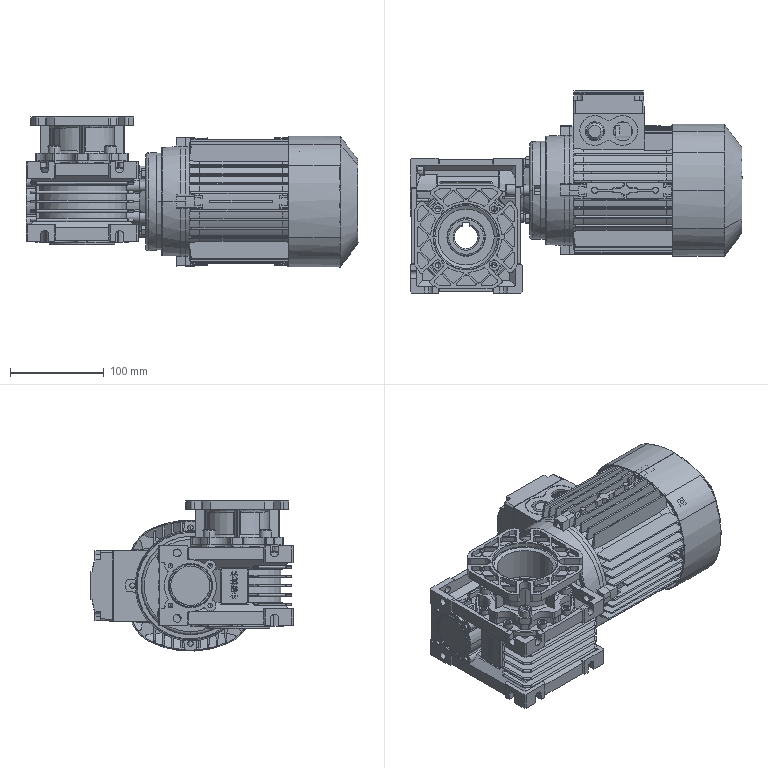Part | SolidWorks | features MBimport 1 | 26 solids | 3489 faces | volume 1755237 mm3 | plane 1620 | cylinder 1217 | cone 378 | spline 222 | torus 52 | commonest cylinder face diameters 4 x161 2.5 x115 2 x100 6 x78 1.6 x54 100 x45